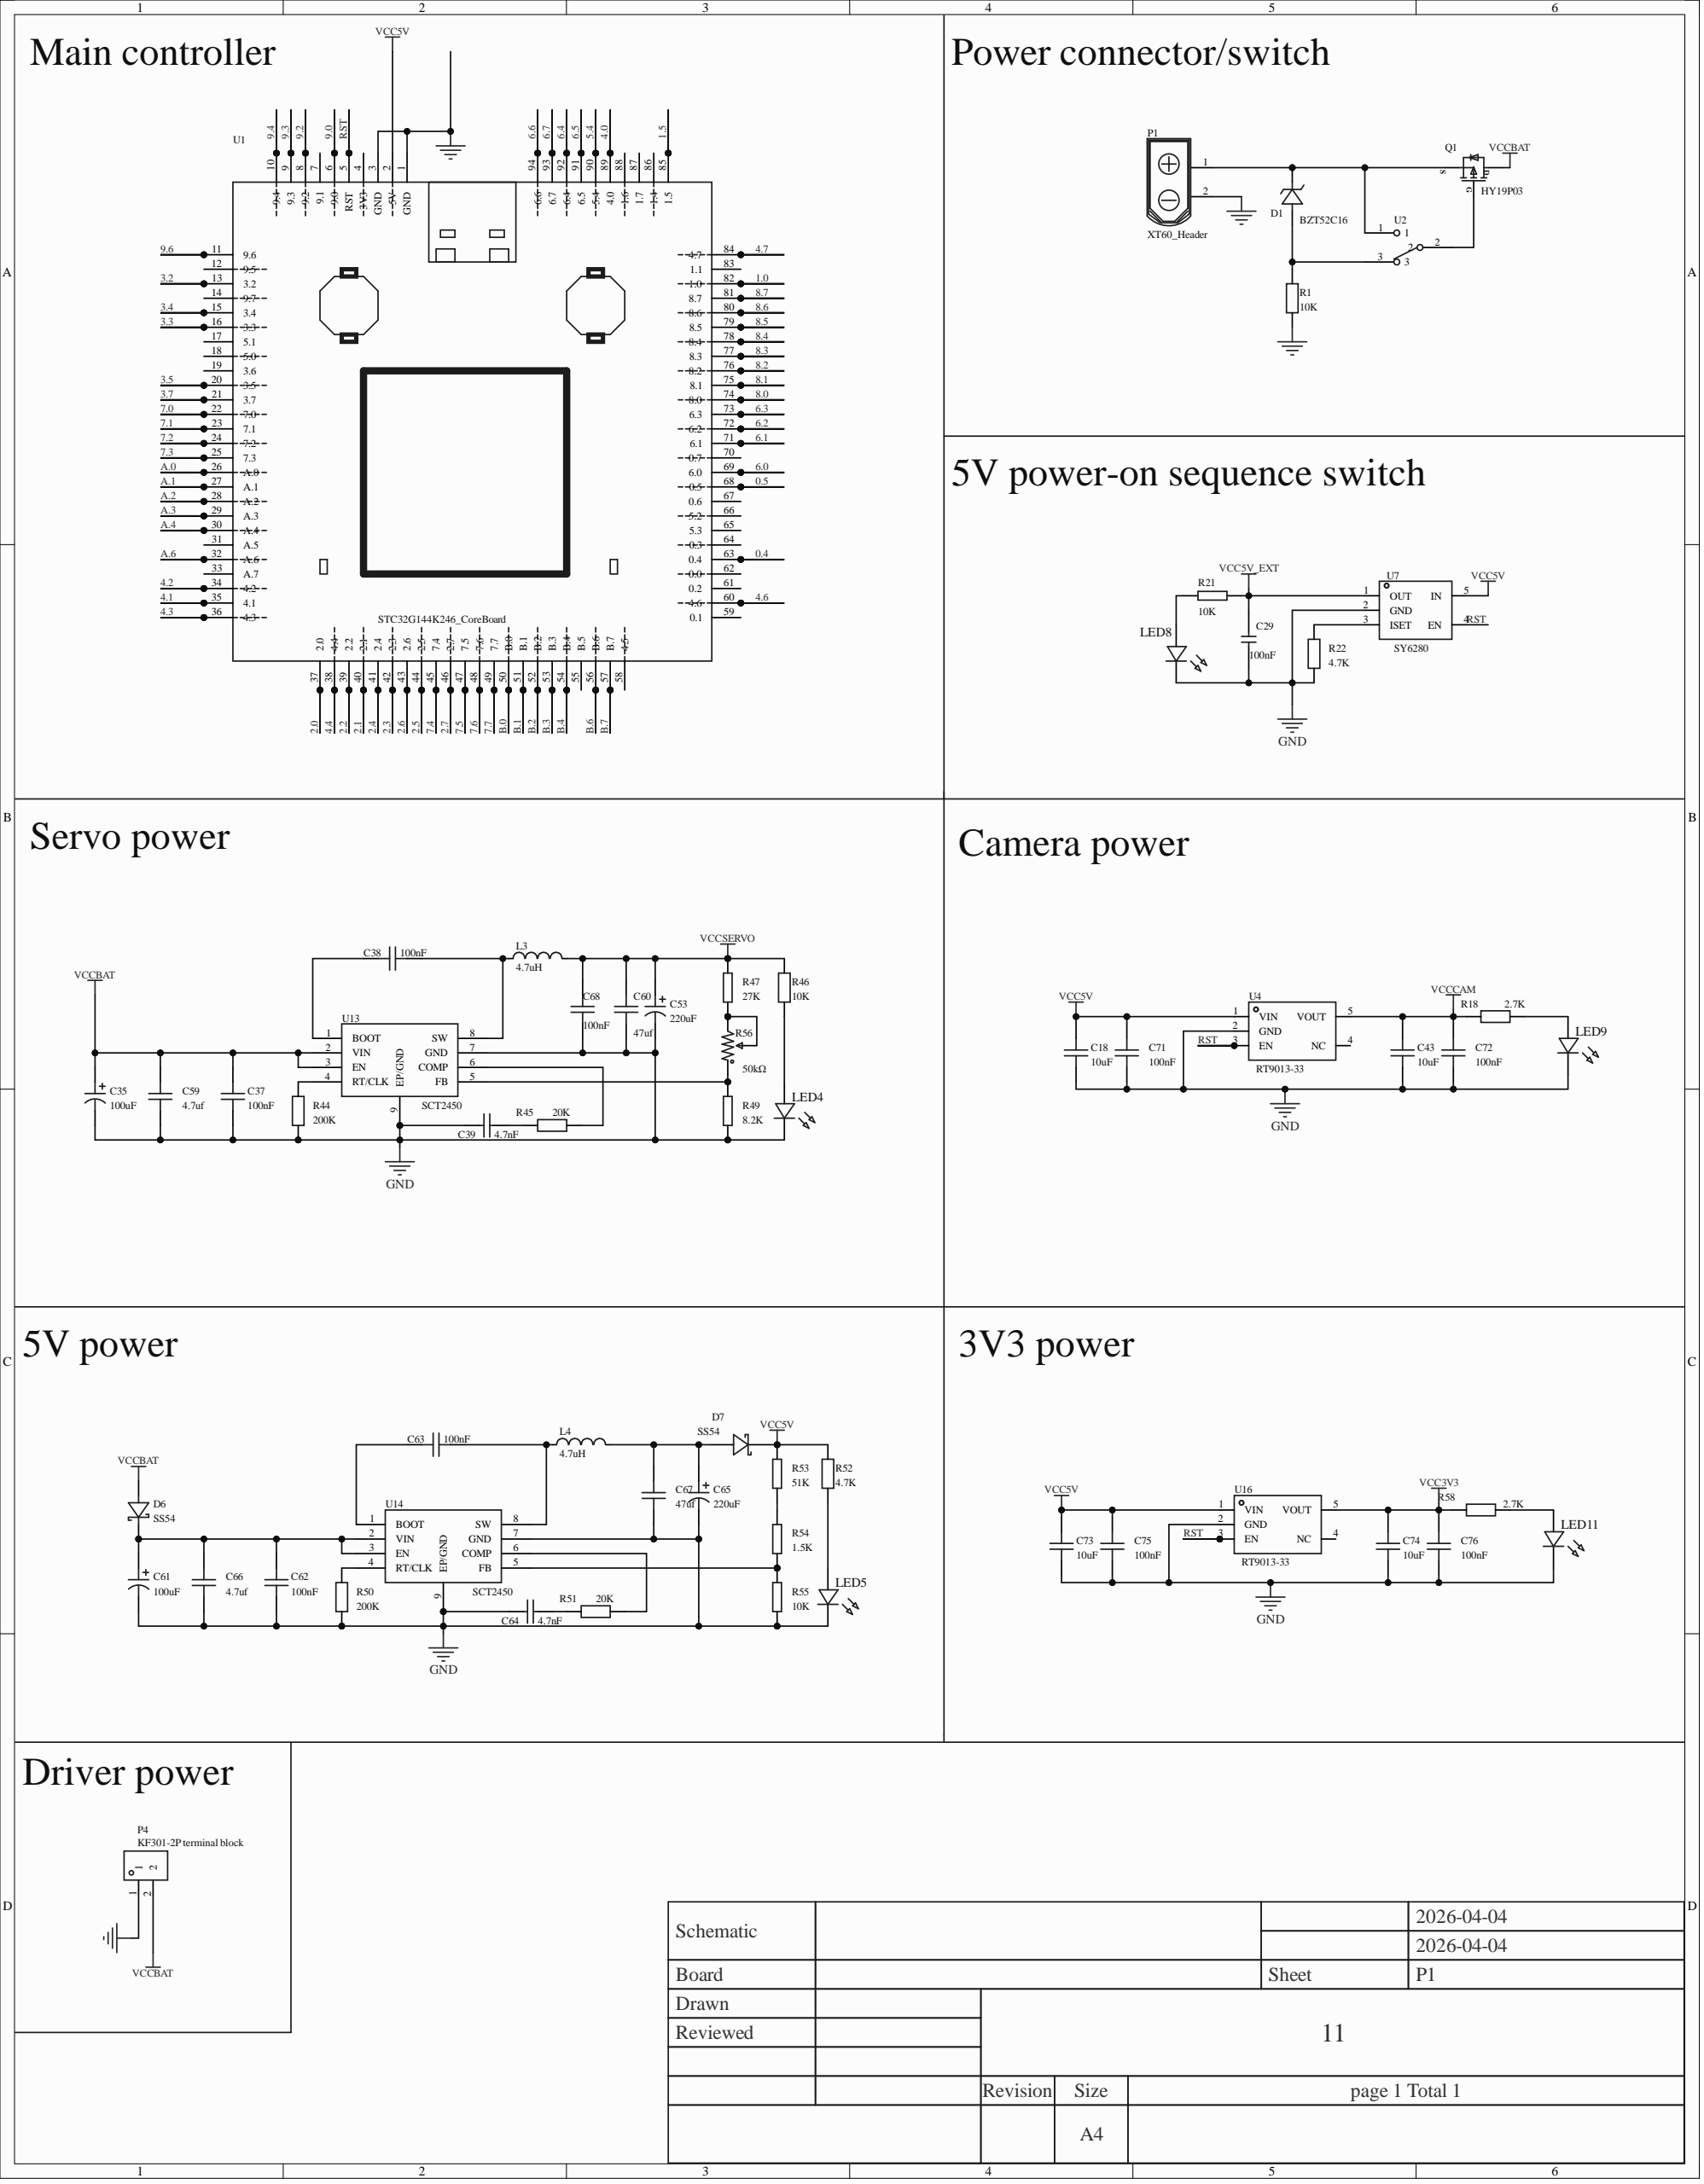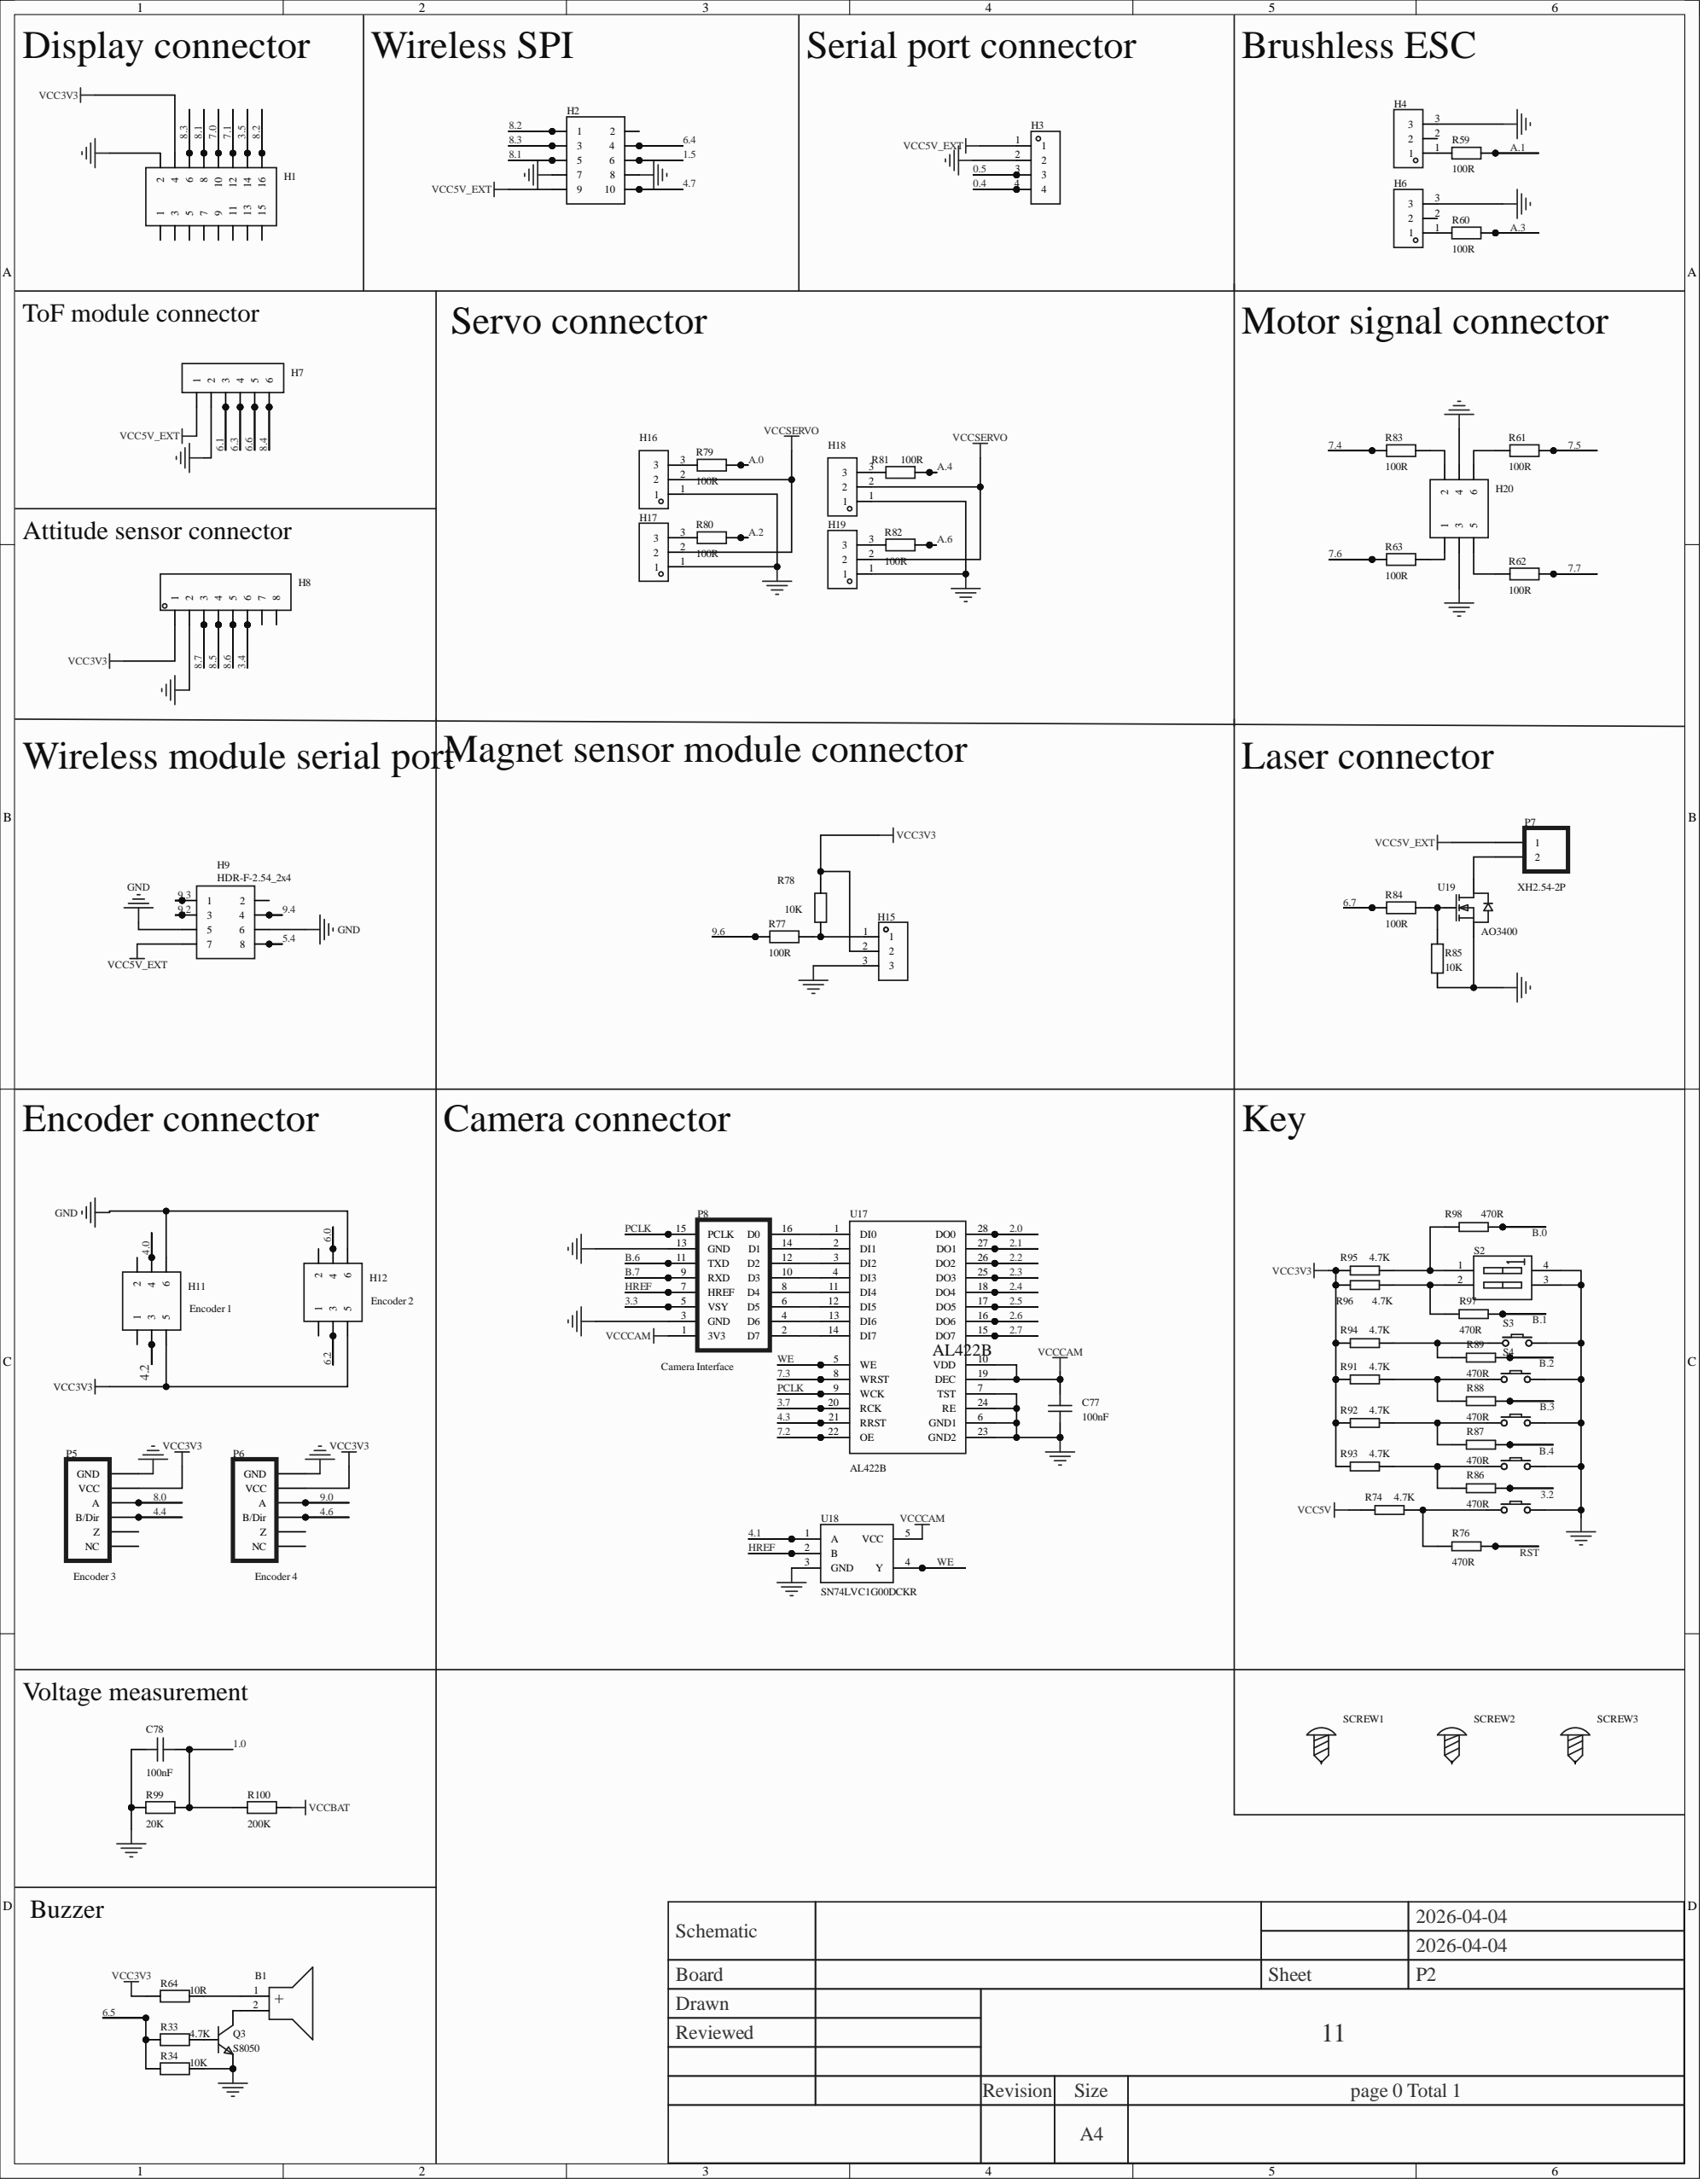Circuit board | Altium Designer | 130 parts | 134 nets
Bill of materials:
Comment,Description,Designator,Footprint,LibRef,Quantity
"3kHz","Drive method: active (built-in driver circuit); Construction: electromagnetic; Frequency: 3kHz; Sound pressure (SPL): 85dB@10cm;","B1","BUZ-TH_BD9.0-P5.00-D0.6-FD","HNB09A03","1"
"10uF","Capacitance: 100nF; Tolerance: ±10%; Rated voltage: 50V; Dielectric (temperature coefficient): X7R;","C18, C43, C73, C74","C0603","CC0603KRX7R9BB104","4"
"100nF","","C29","CAPC1608[0603]S-N","100nF 0603 50V X7R","1"
"100uF","Capacitance: 100uF; Tolerance: ±20%; Rated voltage: 35V; Ripple current: 230mA@120Hz; ESR: 600mΩ@100kHz;","C35, C61","CAP-SMD_BD6.3-L6.6-W6.6-LS7.6-FD-1","RVE100UF35V67RV0072","2"
"100nF","Capacitance: 100nF; Tolerance: ±10%; Rated voltage: 50V; Dielectric (temperature coefficient): X7R;, [NoValue]","C37, C38, C62, C63, C68, C71, C72, C75, C76, C77, C78","C0603","CC0603KRX7R9BB104, CAP_0603","11"
"4.7nF","Capacitance: 4.7nF; Tolerance: ±10%; Rated voltage: 50V; Dielectric (temperature coefficient): X7R;","C39, C64","C0603","0603B472K500NT","2"
"220uF","Capacitance: 100uF; Tolerance: ±20%; Rated voltage: 35V; Ripple current: 230mA@120Hz; ESR: 600mΩ@100kHz;","C53, C65","CAP-SMD_BD6.3-L6.6-W6.6-LS7.6-FD-1","RVE100UF35V67RV0072","2"
"4.7uf","","C59, C66","C1206","CAP_1206","2"
"47uf","","C60, C67","C1206","CAP_1206","2"
"BZT52C16","Zener voltage (nominal): -; Power: 500mW; Tolerance: -;","D1","SOD-123_L2.7-W1.6-LS3.7-RD","BZT52C16","1"
"SS54","Diode configuration: single; Forward voltage (Vf): 550mV@5.0A; DC reverse voltage (Vr): 40V; Average rectified current (Io): 5A;","D6","SMA_L4.3-W2.6-LS5.0-FD","SS54_C7420369","1"
"SS54","","D7","SMA-L[DO-214AC]","SS54","1"
"","","H1","HDR-TH_16P-P2.54-V-F-R2-C8-S2.54-1","HDR-F_2.54_2x8","1"
"","","H2","HDR-TH_10P-P2.54-V-F-R2-C5-S2.54","HDR-F_2.54_2x5","1"
"","","H3","HDR-TH_4P-P2.54-V-M","HDR-M_2.54_1x4P","1"
"","","H4, H6, H15, H16, H17, H18, H19","HDR-TH_3P-P2.54-V-M","HDR-M_2.54_1x3P","7"
"","","H7","HDR-TH_6P-P2.54-V-M-1","HDR-M_2.54_1x6P","1"
"","","H8","HDR-TH_8P-P2.54-V-M","HDR-M_2.54_1x8P","1"
"HDR-F-2.54_2x4","","H9","HDR-F-2.54_2X4","HDR-F-2.54_2x4","1"
"","","H11, H12, H20","HDR-TH_6P-P2.54-V-R2-C3-S2.54_A2541WV-2X3P","HDR-M_2.54_2x3","3"
"4.7uH","Inductance: 4.7uH; Tolerance: ±20%; Rated current: 5A; DC resistance (DCR): 34.5mΩ;","L3, L4","IND-SMD_L7.2-W6.6_GPSR07X0","CYA0630-4.7UH","2"
"","","LED4, LED5, LED8, LED9, LED11","LED_0603","LED_0603-R","5"
"XT60_Header","","P1","Wired T-Header ThroughHole","XT60_Header","1"
"KF301-2P terminal block","","P4","CONN-TH_XY301V-A-5.0-2P","KF301-2P接线端子","1"
"GH1.25-6P-SH new encoder board end, horizontal","Seekfree 1024-line encoder GH1.25-6P mainboard end, horizontal","P5, P6","ECD-GH1.25-6P-SV","GH1.25-6P-SH新编码器主板端-卧式","2"
"XH2.54-2P","XH2.54-2P","P7","XH2.54-2P-DV","XH2.54-2P","1"
"Camera Interface","Camera adapter board connector 2x8 dual-row socket","P8","HDR2X8-F-High","Camera Interface","1"
"HY19P03","","Q1","TO-252AA","HY19P03","1"
"S8050","Transistor type: NPN; Collector current (Ic): 500mA; Collector-emitter breakdown voltage (Vceo): 25V; Power (Pd): 300mW; DC current gain (hFE@Ic,Vce): 200@50mA,1V;","Q3","SOT-23-3_L3.0-W1.7-P0.95-LS2.9-BR","S8050 J3Y_C2146","1"
"10K","","R1, R34, R46, R78, R85","R0603","Res_0603","5"
"2.7K","","R18, R58","R0603","Res_0603","2"
"10K","","R21, R55","RESC1608[0603]S-N","Res-Chip","2"
"4.7K","","R22, R33, R52","R0603","Res_0603","3"
"200K","","R44, R50, R100","R0603","Res_0603","3"
"20K","","R45, R51, R99","R0603","Res_0603","3"
"27K","","R47","RESC1608[0603]S-N","Res-Chip_6","1"
"8.2K","","R49","RESC1608[0603]S-N","Res-Chip","1"
"51K","","R53","RESC1608[0603]S-N","Res-Chip_6","1"
"1.5K","","R54","RESC1608[0603]S-N","Res-Chip_7","1"
"50kΩ","Resistance: 50kΩ; Tolerance: ±10%; Power: 500mW; Temperature coefficient: ±250ppm/?;","R56","RES-ADJ-TH_3P-L9.5-W4.85-P2.50-BL-BS","3296W-1-503_C48997928","1"
"100R","","R59, R60, R61, R62, R63, R77, R79, R80, R81, R82, R83, R84","R0603","Res_0603","12"
"10R","","R64","R0603","Res_0603","1"
"4.7K","","R74, R91, R92, R93, R94, R95, R96","RESC1608[0603]S-N","Res-Chip_5","7"
"470R","","R76, R86, R87, R88, R89, R97, R98","RESC1608[0603]S-N","Res-Chip_5","7"
"SW DIP-2","","S2","Code SW-2-DIP-2.54","Code SW-2","1"
"KEY-TS1145","","S3, S4, S5, S6, S7","TS-1199A","KEY-TS1145","5"
"","","SCREW1, SCREW2, SCREW3","M3螺丝","M3螺丝","3"
"STC32G144K246_CoreBoard","STC32G144K246_Core Seekfree STC32G144K246 core board","U1","STC32G144K246_CoreBoard","STC32G144K246_CoreBoard","1"
"","","U2","SS12D10","kaiguan","1"
"RT9013-33","Output type: fixed; Max input voltage: 5.5V; Output voltage: 3.3V; Max output current: 500mA; Power supply rejection ratio (PSRR): 50dB@(10kHz); Output polarity: positive;","U4, U16","SOT-23-5","RT9013-33GU5","2"
"SY6280","Low-power distribution switch","U7","SOT-23-5_L3.0-W1.7-P0.95-LS2.8-BL","SY6280AAC_C55136","1"
"SCT2450","","U13, U14","SOP-8E","SCT2450","2"
"AL422B","8-channel FIFO memory","U17","SOP-28","AL422B","1"
"SN74LVC1G00DCKR","SN74LVC1G00DCKR NAND gate","U18","SOT-353","SN74LVC1G00DCKR","1"
"AO3400","","U19","SOT-23-3_L2.9-W1.3-P1.90-LS2.4-BL-2","AO3400","1"
Netlist (Protel format):
[
B1
BUZ-TH_BD9.0-P5.00-D0.6-FD
3kHz



]
[
C18
C0603
10uF



]
[
C29
CAPC1608[0603]S-N
100nF



]
[
C35
CAP-SMD_BD6.3-L6.6-W6.6-LS7.6-FD-1
100uF



]
[
C37
C0603
100nF



]
[
C38
C0603
100nF



]
[
C39
C0603
4.7nF



]
[
C43
C0603
10uF



]
[
C53
CAP-SMD_BD6.3-L6.6-W6.6-LS7.6-FD-1
220uF



]
[
C59
C1206
4.7uf



]
[
C60
C1206
47uf



]
[
C61
CAP-SMD_BD6.3-L6.6-W6.6-LS7.6-FD-1
100uF



]
[
C62
C0603
100nF



]
[
C63
C0603
100nF



]
[
C64
C0603
4.7nF



]
[
C65
CAP-SMD_BD6.3-L6.6-W6.6-LS7.6-FD-1
220uF



]
[
C66
C1206
4.7uf



]
[
C67
C1206
47uf



]
[
C68
C0603
100nF



]
[
C71
C0603
100nF



]
[
C72
C0603
100nF



]
[
C73
C0603
10uF



]
[
C74
C0603
10uF



]
[
C75
C0603
100nF



]
[
C76
C0603
100nF



]
[
C77
C0603
100nF



]
[
C78
C0603
100nF



]
[
D1
SOD-123_L2.7-W1.6-LS3.7-RD
BZT52C16



]
[
D6
SMA_L4.3-W2.6-LS5.0-FD
SS54



]
[
D7
SMA-L[DO-214AC]
SS54



]
[
H1
HDR-TH_16P-P2.54-V-F-R2-C8-S2.54-1




]
[
H2
HDR-TH_10P-P2.54-V-F-R2-C5-S2.54




]
[
H3
HDR-TH_4P-P2.54-V-M




]
[
H4
HDR-TH_3P-P2.54-V-M




]
[
H6
HDR-TH_3P-P2.54-V-M




]
[
H7
HDR-TH_6P-P2.54-V-M-1




]
[
H8
HDR-TH_8P-P2.54-V-M




]
[
H9
HDR-F-2.54_2X4
HDR-F-2.54_2x4



]
[
H11
HDR-TH_6P-P2.54-V-R2-C3-S2.54_A2541WV-2X3P




]
[
H12
HDR-TH_6P-P2.54-V-R2-C3-S2.54_A2541WV-2X3P




]
[
H15
HDR-TH_3P-P2.54-V-M




]
[
H16
HDR-TH_3P-P2.54-V-M




]
[
H17
HDR-TH_3P-P2.54-V-M




]
[
H18
HDR-TH_3P-P2.54-V-M




]
[
H19
HDR-TH_3P-P2.54-V-M




]
[
H20
HDR-TH_6P-P2.54-V-R2-C3-S2.54_A2541WV-2X3P




]
[
L3
IND-SMD_L7.2-W6.6_GPSR07X0
4.7uH



]
[
L4
IND-SMD_L7.2-W6.6_GPSR07X0
4.7uH



]
[
LED4
LED_0603




]
[
LED5
LED_0603




]
[
LED8
LED_0603




]
[
LED9
LED_0603




]
[
LED11
LED_0603




]
[
P1
Wired T-Header ThroughHole
XT60_Header



]
[
P4
CONN-TH_XY301V-A-5.0-2P
KF301-2P terminal block



]
[
P5
ECD-GH1.25-6P-SV
GH1.25-6P-SH new encoder board end, horizontal



]
[
P6
ECD-GH1.25-6P-SV
GH1.25-6P-SH new encoder board end, horizontal



]
[
P7
XH2.54-2P-DV
XH2.54-2P



]
[
P8
HDR2X8-F-High
Camera Interface



]
[
Q1
TO-252AA
HY19P03



]
[
Q3
SOT-23-3_L3.0-W1.7-P0.95-LS2.9-BR
S8050



]
[
R1
R0603
10K



]
[
R18
R0603
2.7K



]
[
R21
RESC1608[0603]S-N
10K



]
[
R22
R0603
4.7K



]
[
R33
R0603
4.7K



]
[
R34
R0603
10K



]
[
R44
R0603
200K



]
[
R45
R0603
20K



]
[
R46
R0603
10K



]
[
R47
RESC1608[0603]S-N
27K



]
[
R49
RESC1608[0603]S-N
8.2K



]
[
R50
R0603
200K



]
[
R51
R0603
20K



]
[
R52
R0603
4.7K



]
[
R53
RESC1608[0603]S-N
51K



]
[
R54
RESC1608[0603]S-N
1.5K



]
[
R55
RESC1608[0603]S-N
10K



]
[
R56
RES-ADJ-TH_3P-L9.5-W4.85-P2.50-BL-BS
50kΩ



]
[
R58
R0603
2.7K



]
[
R59
R0603
100R



]
[
R60
R0603
100R



]
[
R61
R0603
100R



]
[
R62
R0603
100R



]
[
R63
R0603
100R



]
[
R64
R0603
10R



]
[
R74
RESC1608[0603]S-N
4.7K



]
[
R76
RESC1608[0603]S-N
470R



]
[
R77
R0603
100R



]
[
R78
R0603
10K



]
[
R79
R0603
100R



]
[
R80
R0603
100R



]
[
R81
R0603
100R



]
[
R82
R0603
100R



]
[
R83
R0603
100R



]
[
R84
R0603
100R



]
[
R85
R0603
10K



]
[
R86
RESC1608[0603]S-N
470R



]
[
R87
RESC1608[0603]S-N
470R



]
[
R88
RESC1608[0603]S-N
470R



]
[
R89
RESC1608[0603]S-N
470R



]
[
R91
RESC1608[0603]S-N
4.7K



]
[
R92
RESC1608[0603]S-N
4.7K



]
[
R93
RESC1608[0603]S-N
4.7K



]
[
R94
RESC1608[0603]S-N
4.7K



]
[
R95
RESC1608[0603]S-N
4.7K



]
[
R96
RESC1608[0603]S-N
4.7K



]
[
R97
RESC1608[0603]S-N
470R



]
[
R98
RESC1608[0603]S-N
470R



]
[
R99
R0603
20K



]
[
R100
R0603
200K



]
[
S2
Code SW-2-DIP-2.54
SW DIP-2



]
[
S3
TS-1199A
KEY-TS1145



]
[
S4
TS-1199A
KEY-TS1145



]
[
S5
TS-1199A
KEY-TS1145



]
[
S6
TS-1199A
KEY-TS1145



]
[
S7
TS-1199A
KEY-TS1145



]
[
SCREW1
M3螺丝




]
[
SCREW2
M3螺丝




]
[
SCREW3
M3螺丝




]
[
U1
STC32G144K246_CoreBoard
STC32G144K246_CoreBoard



]
[
U2
SS12D10




]
[
U4
SOT-23-5
RT9013-33



]
[
U7
SOT-23-5_L3.0-W1.7-P0.95-LS2.8-BL
SY6280



]
[
U13
SOP-8E
SCT2450



]
[
U14
SOP-8E
SCT2450



]
[
U16
SOT-23-5
RT9013-33



]
[
U17
SOP-28
AL422B



]
[
U18
SOT-353
SN74LVC1G00DCKR



]
[
U19
SOT-23-3_L2.9-W1.3-P1.90-LS2.4-BL-2
AO3400



]
(
WE
U17-5
U18-4
)
(
VCCSERVO
C53-1
C60-2
C68-2
H16-2
H17-2
H18-2
H19-2
L3-2
R46-1
R47-2
)
(
VCCCAM
C43-2
C72-2
C77-2
P8-1
R18-1
U4-5
U17-10
U17-19
U18-5
)
(
VCCBAT
C35-1
C37-2
C59-2
D6-1
P4-2
Q1-1
R100-2
U13-2
U13-3
)
(
VCC5V_EXT
C29-2
H2-9
H3-1
H7-1
H9-7
P7-1
R21-1
U7-1
)
(
VCC5V
C18-2
C71-2
C73-2
C75-2
D7-K
R52-1
R53-2
R74-1
U1-2
U4-1
U7-5
U16-1
)
(
VCC3V3
C74-2
C76-2
H1-4
H8-1
H11-5
H12-5
H15-2
P5-2
P6-2
R58-1
R64-1
R78-2
R91-1
R92-1
R93-1
R94-1
R95-1
R96-1
U16-5
)
(
RST
R76-1
U1-5
U4-3
U7-4
U16-3
)
(
PCLK
P8-15
U17-9
)
(
NetR96_2
R96-2
R97-2
S2-2
)
(
NetR95_2
R95-2
R98-2
S2-1
)
(
NetR89_2
R89-2
R94-2
S3-2
)
(
NetR88_2
R88-2
R91-2
S4-2
)
(
NetR87_2
R87-2
R92-2
S5-2
)
(
NetR86_2
R86-2
R93-2
S6-2
)
(
NetR84_2
R84-2
R85-2
U19-1
)
(
NetR74_2
R74-2
R76-2
S7-2
)
(
NetR54_1
R54-1
R55-2
U14-5
)
(
NetR53_1
R53-1
R54-2
)
(
NetR51_1
R51-1
U14-6
)
(
NetR50_2
R50-2
U14-4
)
(
NetR49_2
R49-2
R56-1
U13-5
)
(
NetR47_1
R47-1
R56-2
R56-3
)
(
NetR45_1
R45-1
U13-6
)
(
NetR44_2
R44-2
U13-4
)
(
NetR22_2
R22-2
U7-3
)
(
NetQ3_1
Q3-1
R33-2
)
(
NetQ1_2
Q1-2
U2-2
)
(
NetP8_16
P8-16
U17-1
)
(
NetP8_14
P8-14
U17-2
)
(
NetP8_12
P8-12
U17-3
)
(
NetP8_10
P8-10
U17-4
)
(
NetP8_8
P8-8
U17-11
)
(
NetP8_6
P8-6
U17-12
)
(
NetP8_4
P8-4
U17-13
)
(
NetP8_2
P8-2
U17-14
)
(
NetP7_2
P7-2
U19-3
)
(
NetLED11_2
LED11-2
R58-2
)
(
NetLED9_2
LED9-2
R18-2
)
(
NetLED8_2
LED8-2
R21-2
)
(
NetLED5_2
LED5-2
R52-2
)
(
NetLED4_2
LED4-2
R46-2
)
(
NetH20_6
H20-6
R61-1
)
(
NetH20_5
H20-5
R62-1
)
(
NetH20_2
H20-2
R83-2
)
(
NetH20_1
H20-1
R63-2
)
(
NetH19_3
H19-3
R82-1
)
(
NetH18_3
H18-3
R81-1
)
(
NetH17_3
H17-3
R80-1
)
(
NetH16_3
H16-3
R79-1
)
(
NetH15_1
H15-1
R77-2
R78-1
)
(
NetH6_1
H6-1
R60-1
)
(
NetH4_1
H4-1
R59-1
)
(
NetD1_2
D1-2
R1-2
U2-3
)
(
NetD1_1
D1-1
P1-1
Q1-3
U2-1
)
(
NetC65_1
C65-1
C67-2
D7-A
L4-2
)
(
NetC64_2
C64-2
R51-2
)
(
NetC63_2
C63-2
U14-1
)
(
NetC63_1
C63-1
L4-1
U14-8
)
(
NetC61_1
C61-1
C62-2
C66-2
D6-2
U14-2
U14-3
)
(
NetC39_2
C39-2
R45-2
)
(
NetC38_2
C38-2
U13-1
)
(
NetC38_1
C38-1
L3-1
U13-8
)
(
NetB1_2
B1-2
Q3-3
)
(
NetB1_1
B1-1
R64-2
)
(
HREF
P8-7
U18-2
)
(
GND
C18-1
C29-1
C35-2
C37-1
C39-1
C43-1
C53-2
C59-1
C60-1
C61-2
C62-1
C64-1
C65-2
C66-1
C67-1
C68-1
C71-1
C72-1
C73-1
C74-1
C75-1
C76-1
C77-1
C78-1
H1-2
H2-7
H2-8
H3-2
H4-3
H6-3
H7-2
H8-2
H9-5
H9-6
H11-6
H12-6
H15-3
H16-1
H17-1
H18-1
H19-1
H20-3
H20-4
LED4-1
LED5-1
LED8-1
LED9-1
LED11-1
P1-2
P4-1
P5-1
P6-1
P8-3
P8-13
Q3-2
R1-1
R22-1
R34-2
R44-1
R49-1
R50-1
R55-1
R85-1
R99-1
S2-3
S2-4
S3-1
S4-1
S5-1
S6-1
S7-1
U1-1
U1-3
U4-2
U7-2
U13-7
U13-9
U14-7
U14-9
U16-2
U17-6
U17-7
U17-23
U17-24
U18-3
U19-2
)
(
B.7
P8-9
U1-57
)
(
B.6
P8-11
U1-56
)
(
B.4
R87-1
U1-54
)
(
B.3
R88-1
U1-53
)
(
B.2
R89-1
U1-52
)
(
B.1
R97-1
U1-51
)
(
B.0
R98-1
U1-50
)
(
A.6
R82-2
U1-32
)
(
A.4
R81-2
U1-30
)
(
A.3
R60-2
U1-29
)
(
A.2
R80-2
U1-28
)
(
A.1
R59-2
U1-27
)
(
A.0
R79-2
U1-26
)
(
9.6
R77-1
U1-11
)
(
9.4
H9-4
U1-10
)
(
9.3
H9-1
U1-9
)
(
9.2
H9-3
U1-8
)
(
9.0
P6-3
U1-6
)
(
8.7
H8-3
U1-81
)
(
8.6
H8-5
U1-80
)
(
8.5
H8-4
U1-79
)
(
8.4
H7-6
U1-78
)
(
8.3
H1-6
H2-3
U1-77
)
(
8.2
H1-16
H2-1
U1-76
)
(
8.1
H1-8
H2-5
U1-75
)
(
8.0
P5-3
U1-74
)
(
7.7
R62-2
U1-49
)
(
7.6
R63-1
U1-48
)
(
7.5
R61-2
U1-47
)
(
7.4
R83-1
U1-45
)
(
7.3
U1-25
U17-8
)
(
7.2
U1-24
U17-22
)
(
7.1
H1-12
U1-23
)
(
7.0
H1-10
U1-22
)
(
6.7
R84-1
U1-93
)
(
6.6
H7-5
U1-94
)
(
6.5
R33-1
R34-1
U1-91
)
(
6.4
H2-4
U1-92
)
(
6.3
H7-4
U1-73
)
(
6.2
H12-3
U1-72
)
(
6.1
H7-3
U1-71
)
(
6.0
H12-4
U1-69
)
(
5.4
H9-8
U1-90
)
(
4.7
H2-10
U1-84
)
(
4.6
P6-4
U1-60
)
(
4.4
P5-4
U1-38
)
(
4.3
U1-36
U17-21
)
(
4.2
H11-3
U1-34
)
(
4.1
U1-35
U18-1
)
(
4.0
H11-4
U1-89
)
(
3.7
U1-21
U17-20
)
(
3.5
H1-14
U1-20
)
(
3.4
H8-6
U1-15
)
(
3.3
P8-5
U1-16
)
(
3.2
R86-1
U1-13
)
(
2.7
U1-46
U17-15
)
(
2.6
U1-43
U17-16
)
(
2.5
U1-44
U17-17
)
(
2.4
U1-41
U17-18
)
(
2.3
U1-42
U17-25
)
(
2.2
U1-39
U17-26
)
(
2.1
U1-40
U17-27
)
(
2.0
U1-37
U17-28
)
(
1.5
H2-6
U1-85
)
(
1.0
C78-2
R99-2
R100-1
U1-82
)
(
0.5
H3-3
U1-68
)
(
0.4
H3-4
U1-63
)